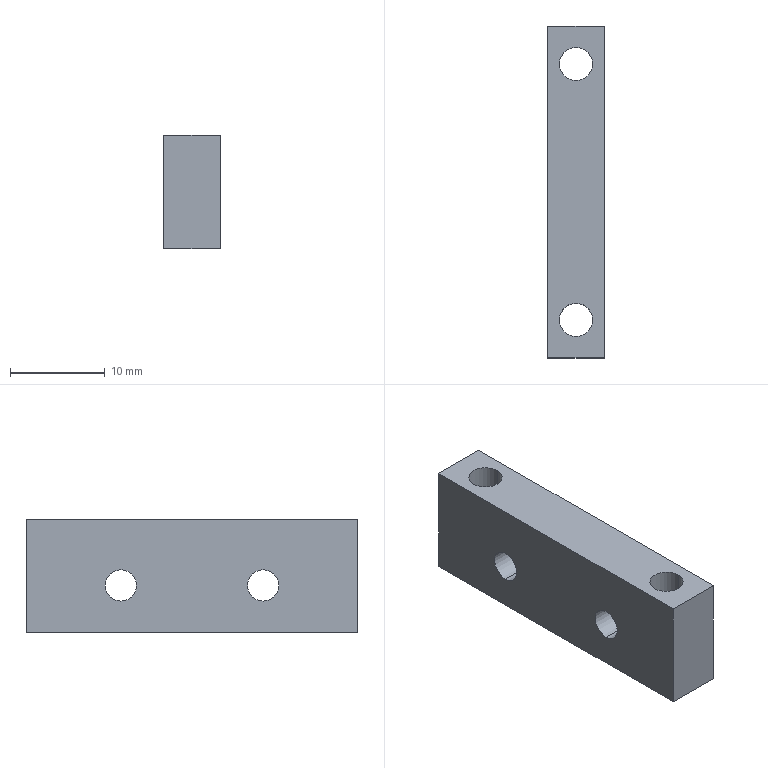Part | STEP file | Belt tensioner seat 1001 | 1 solid | 14 faces | box 6 x 35 x 12 mm | volume 2186 mm3 | cylinder 8 | plane 6 | commonest cylinder face diameters 3.3 x4 3.5 x4
STEP:
#1=CARTESIAN_POINT('',(0.,0.,0.));
#2=DIRECTION('',(0.,0.,1.));
#3=DIRECTION('',(1.,0.,0.));
#4=AXIS2_PLACEMENT_3D('',#1,#2,#3);
#5=CARTESIAN_POINT('',(0.,7.5,-8.65));
#6=VERTEX_POINT('',#5);
#7=CARTESIAN_POINT('',(6.,7.5,-8.65));
#8=VERTEX_POINT('',#7);
#9=CARTESIAN_POINT('',(6.,7.5,-8.65));
#10=DIRECTION('',(1.,0.,0.));
#11=VECTOR('',#10,1.);
#12=LINE('',#9,#11);
#13=CARTESIAN_POINT('',(6.,7.5,-7.));
#14=DIRECTION('',(1.,0.,0.));
#15=DIRECTION('',(0.,0.,-1.));
#16=AXIS2_PLACEMENT_3D('',#13,#14,#15);
#17=CYLINDRICAL_SURFACE('',#16,1.65);
#18=CARTESIAN_POINT('',(6.283,0.));
#19=DIRECTION('',(0.,1.));
#20=VECTOR('',#19,1.);
#21=LINE('',#18,#20);
#22=(GEOMETRIC_REPRESENTATION_CONTEXT(2)PARAMETRIC_REPRESENTATION_CONTEXT()REPRESENTATION_CONTEXT('',''));
#23=DEFINITIONAL_REPRESENTATION('',(#21),#22);
#24=PCURVE('',#17,#23);
#25=CARTESIAN_POINT('',(6.,7.5,-7.));
#26=DIRECTION('',(1.,0.,0.));
#27=DIRECTION('',(0.,0.,-1.));
#28=AXIS2_PLACEMENT_3D('',#25,#26,#27);
#29=CYLINDRICAL_SURFACE('',#28,1.65);
#30=CARTESIAN_POINT('',(0.,0.));
#31=DIRECTION('',(0.,1.));
#32=VECTOR('',#31,1.);
#33=LINE('',#30,#32);
#34=(GEOMETRIC_REPRESENTATION_CONTEXT(2)PARAMETRIC_REPRESENTATION_CONTEXT()REPRESENTATION_CONTEXT('',''));
#35=DEFINITIONAL_REPRESENTATION('',(#33),#34);
#36=PCURVE('',#29,#35);
#37=SURFACE_CURVE('',#12,(#24,#36),.PCURVE_S1.);
#38=EDGE_CURVE('',#6,#8,#37,.T.);
#39=ORIENTED_EDGE('',*,*,#38,.T.);
#40=CARTESIAN_POINT('',(6.,7.5,-5.35));
#41=VERTEX_POINT('',#40);
#42=CARTESIAN_POINT('',(6.,7.5,-7.));
#43=DIRECTION('',(1.,0.,0.));
#44=DIRECTION('',(0.,0.,-1.));
#45=AXIS2_PLACEMENT_3D('',#42,#43,#44);
#46=CIRCLE('',#45,1.65);
#47=CARTESIAN_POINT('',(0.,0.));
#48=DIRECTION('',(1.,0.));
#49=VECTOR('',#48,1.);
#50=LINE('',#47,#49);
#51=(GEOMETRIC_REPRESENTATION_CONTEXT(2)PARAMETRIC_REPRESENTATION_CONTEXT()REPRESENTATION_CONTEXT('',''));
#52=DEFINITIONAL_REPRESENTATION('',(#50),#51);
#53=PCURVE('',#17,#52);
#54=CARTESIAN_POINT('',(6.,17.5,-12.));
#55=DIRECTION('',(1.,0.,0.));
#56=DIRECTION('',(0.,0.,-1.));
#57=AXIS2_PLACEMENT_3D('',#54,#55,#56);
#58=PLANE('',#57);
#59=CARTESIAN_POINT('',(-5.,-10.));
#60=DIRECTION('',(1.,0.));
#61=AXIS2_PLACEMENT_2D('',#59,#60);
#62=CIRCLE('',#61,1.65);
#63=(GEOMETRIC_REPRESENTATION_CONTEXT(2)PARAMETRIC_REPRESENTATION_CONTEXT()REPRESENTATION_CONTEXT('',''));
#64=DEFINITIONAL_REPRESENTATION('',(#62),#63);
#65=PCURVE('',#58,#64);
#66=SURFACE_CURVE('',#46,(#53,#65),.PCURVE_S1.);
#67=EDGE_CURVE('',#41,#8,#66,.T.);
#68=ORIENTED_EDGE('',*,*,#67,.F.);
#69=CARTESIAN_POINT('',(0.,7.5,-5.35));
#70=VERTEX_POINT('',#69);
#71=CARTESIAN_POINT('',(6.,7.5,-5.35));
#72=DIRECTION('',(1.,0.,0.));
#73=VECTOR('',#72,1.);
#74=LINE('',#71,#73);
#75=CARTESIAN_POINT('',(3.142,0.));
#76=DIRECTION('',(0.,1.));
#77=VECTOR('',#76,1.);
#78=LINE('',#75,#77);
#79=(GEOMETRIC_REPRESENTATION_CONTEXT(2)PARAMETRIC_REPRESENTATION_CONTEXT()REPRESENTATION_CONTEXT('',''));
#80=DEFINITIONAL_REPRESENTATION('',(#78),#79);
#81=PCURVE('',#17,#80);
#82=CARTESIAN_POINT('',(3.142,0.));
#83=DIRECTION('',(0.,1.));
#84=VECTOR('',#83,1.);
#85=LINE('',#82,#84);
#86=(GEOMETRIC_REPRESENTATION_CONTEXT(2)PARAMETRIC_REPRESENTATION_CONTEXT()REPRESENTATION_CONTEXT('',''));
#87=DEFINITIONAL_REPRESENTATION('',(#85),#86);
#88=PCURVE('',#29,#87);
#89=SURFACE_CURVE('',#74,(#81,#88),.PCURVE_S1.);
#90=EDGE_CURVE('',#70,#41,#89,.T.);
#91=ORIENTED_EDGE('',*,*,#90,.F.);
#92=CARTESIAN_POINT('',(0.,7.5,-7.));
#93=DIRECTION('',(-1.,0.,0.));
#94=DIRECTION('',(0.,0.,1.));
#95=AXIS2_PLACEMENT_3D('',#92,#93,#94);
#96=CIRCLE('',#95,1.65);
#97=CARTESIAN_POINT('',(9.425,-6.));
#98=DIRECTION('',(-1.,0.));
#99=VECTOR('',#98,1.);
#100=LINE('',#97,#99);
#101=(GEOMETRIC_REPRESENTATION_CONTEXT(2)PARAMETRIC_REPRESENTATION_CONTEXT()REPRESENTATION_CONTEXT('',''));
#102=DEFINITIONAL_REPRESENTATION('',(#100),#101);
#103=PCURVE('',#17,#102);
#104=CARTESIAN_POINT('',(0.,17.5,0.));
#105=DIRECTION('',(-1.,0.,0.));
#106=DIRECTION('',(0.,0.,1.));
#107=AXIS2_PLACEMENT_3D('',#104,#105,#106);
#108=PLANE('',#107);
#109=CARTESIAN_POINT('',(-7.,-10.));
#110=DIRECTION('',(1.,0.));
#111=AXIS2_PLACEMENT_2D('',#109,#110);
#112=CIRCLE('',#111,1.65);
#113=(GEOMETRIC_REPRESENTATION_CONTEXT(2)PARAMETRIC_REPRESENTATION_CONTEXT()REPRESENTATION_CONTEXT('',''));
#114=DEFINITIONAL_REPRESENTATION('',(#112),#113);
#115=PCURVE('',#108,#114);
#116=SURFACE_CURVE('',#96,(#103,#115),.PCURVE_S1.);
#117=EDGE_CURVE('',#6,#70,#116,.T.);
#118=ORIENTED_EDGE('',*,*,#117,.F.);
#119=EDGE_LOOP('',(#39,#68,#91,#118));
#120=FACE_BOUND('',#119,.F.);
#121=ADVANCED_FACE('',(#120),#17,.F.);
#122=CARTESIAN_POINT('',(0.,-7.5,-8.65));
#123=VERTEX_POINT('',#122);
#124=CARTESIAN_POINT('',(6.,-7.5,-8.65));
#125=VERTEX_POINT('',#124);
#126=CARTESIAN_POINT('',(6.,-7.5,-8.65));
#127=DIRECTION('',(1.,0.,0.));
#128=VECTOR('',#127,1.);
#129=LINE('',#126,#128);
#130=CARTESIAN_POINT('',(6.,-7.5,-7.));
#131=DIRECTION('',(1.,0.,0.));
#132=DIRECTION('',(0.,0.,-1.));
#133=AXIS2_PLACEMENT_3D('',#130,#131,#132);
#134=CYLINDRICAL_SURFACE('',#133,1.65);
#135=CARTESIAN_POINT('',(6.283,0.));
#136=DIRECTION('',(0.,1.));
#137=VECTOR('',#136,1.);
#138=LINE('',#135,#137);
#139=(GEOMETRIC_REPRESENTATION_CONTEXT(2)PARAMETRIC_REPRESENTATION_CONTEXT()REPRESENTATION_CONTEXT('',''));
#140=DEFINITIONAL_REPRESENTATION('',(#138),#139);
#141=PCURVE('',#134,#140);
#142=CARTESIAN_POINT('',(6.,-7.5,-7.));
#143=DIRECTION('',(1.,0.,0.));
#144=DIRECTION('',(0.,0.,-1.));
#145=AXIS2_PLACEMENT_3D('',#142,#143,#144);
#146=CYLINDRICAL_SURFACE('',#145,1.65);
#147=CARTESIAN_POINT('',(0.,0.));
#148=DIRECTION('',(0.,1.));
#149=VECTOR('',#148,1.);
#150=LINE('',#147,#149);
#151=(GEOMETRIC_REPRESENTATION_CONTEXT(2)PARAMETRIC_REPRESENTATION_CONTEXT()REPRESENTATION_CONTEXT('',''));
#152=DEFINITIONAL_REPRESENTATION('',(#150),#151);
#153=PCURVE('',#146,#152);
#154=SURFACE_CURVE('',#129,(#141,#153),.PCURVE_S1.);
#155=EDGE_CURVE('',#123,#125,#154,.T.);
#156=ORIENTED_EDGE('',*,*,#155,.T.);
#157=CARTESIAN_POINT('',(6.,-7.5,-5.35));
#158=VERTEX_POINT('',#157);
#159=CARTESIAN_POINT('',(6.,-7.5,-7.));
#160=DIRECTION('',(1.,0.,0.));
#161=DIRECTION('',(0.,0.,-1.));
#162=AXIS2_PLACEMENT_3D('',#159,#160,#161);
#163=CIRCLE('',#162,1.65);
#164=CARTESIAN_POINT('',(0.,0.));
#165=DIRECTION('',(1.,0.));
#166=VECTOR('',#165,1.);
#167=LINE('',#164,#166);
#168=(GEOMETRIC_REPRESENTATION_CONTEXT(2)PARAMETRIC_REPRESENTATION_CONTEXT()REPRESENTATION_CONTEXT('',''));
#169=DEFINITIONAL_REPRESENTATION('',(#167),#168);
#170=PCURVE('',#134,#169);
#171=CARTESIAN_POINT('',(-5.,-25.));
#172=DIRECTION('',(1.,0.));
#173=AXIS2_PLACEMENT_2D('',#171,#172);
#174=CIRCLE('',#173,1.65);
#175=(GEOMETRIC_REPRESENTATION_CONTEXT(2)PARAMETRIC_REPRESENTATION_CONTEXT()REPRESENTATION_CONTEXT('',''));
#176=DEFINITIONAL_REPRESENTATION('',(#174),#175);
#177=PCURVE('',#58,#176);
#178=SURFACE_CURVE('',#163,(#170,#177),.PCURVE_S1.);
#179=EDGE_CURVE('',#158,#125,#178,.T.);
#180=ORIENTED_EDGE('',*,*,#179,.F.);
#181=CARTESIAN_POINT('',(0.,-7.5,-5.35));
#182=VERTEX_POINT('',#181);
#183=CARTESIAN_POINT('',(6.,-7.5,-5.35));
#184=DIRECTION('',(1.,0.,0.));
#185=VECTOR('',#184,1.);
#186=LINE('',#183,#185);
#187=CARTESIAN_POINT('',(3.142,0.));
#188=DIRECTION('',(0.,1.));
#189=VECTOR('',#188,1.);
#190=LINE('',#187,#189);
#191=(GEOMETRIC_REPRESENTATION_CONTEXT(2)PARAMETRIC_REPRESENTATION_CONTEXT()REPRESENTATION_CONTEXT('',''));
#192=DEFINITIONAL_REPRESENTATION('',(#190),#191);
#193=PCURVE('',#134,#192);
#194=CARTESIAN_POINT('',(3.142,0.));
#195=DIRECTION('',(0.,1.));
#196=VECTOR('',#195,1.);
#197=LINE('',#194,#196);
#198=(GEOMETRIC_REPRESENTATION_CONTEXT(2)PARAMETRIC_REPRESENTATION_CONTEXT()REPRESENTATION_CONTEXT('',''));
#199=DEFINITIONAL_REPRESENTATION('',(#197),#198);
#200=PCURVE('',#146,#199);
#201=SURFACE_CURVE('',#186,(#193,#200),.PCURVE_S1.);
#202=EDGE_CURVE('',#182,#158,#201,.T.);
#203=ORIENTED_EDGE('',*,*,#202,.F.);
#204=CARTESIAN_POINT('',(0.,-7.5,-7.));
#205=DIRECTION('',(-1.,0.,0.));
#206=DIRECTION('',(0.,0.,1.));
#207=AXIS2_PLACEMENT_3D('',#204,#205,#206);
#208=CIRCLE('',#207,1.65);
#209=CARTESIAN_POINT('',(9.425,-6.));
#210=DIRECTION('',(-1.,0.));
#211=VECTOR('',#210,1.);
#212=LINE('',#209,#211);
#213=(GEOMETRIC_REPRESENTATION_CONTEXT(2)PARAMETRIC_REPRESENTATION_CONTEXT()REPRESENTATION_CONTEXT('',''));
#214=DEFINITIONAL_REPRESENTATION('',(#212),#213);
#215=PCURVE('',#134,#214);
#216=CARTESIAN_POINT('',(-7.,-25.));
#217=DIRECTION('',(1.,0.));
#218=AXIS2_PLACEMENT_2D('',#216,#217);
#219=CIRCLE('',#218,1.65);
#220=(GEOMETRIC_REPRESENTATION_CONTEXT(2)PARAMETRIC_REPRESENTATION_CONTEXT()REPRESENTATION_CONTEXT('',''));
#221=DEFINITIONAL_REPRESENTATION('',(#219),#220);
#222=PCURVE('',#108,#221);
#223=SURFACE_CURVE('',#208,(#215,#222),.PCURVE_S1.);
#224=EDGE_CURVE('',#123,#182,#223,.T.);
#225=ORIENTED_EDGE('',*,*,#224,.F.);
#226=EDGE_LOOP('',(#156,#180,#203,#225));
#227=FACE_BOUND('',#226,.F.);
#228=ADVANCED_FACE('',(#227),#134,.F.);
#229=CARTESIAN_POINT('',(4.75,13.5,-12.));
#230=VERTEX_POINT('',#229);
#231=CARTESIAN_POINT('',(4.75,13.5,0.));
#232=VERTEX_POINT('',#231);
#233=CARTESIAN_POINT('',(4.75,13.5,-12.));
#234=DIRECTION('',(0.,0.,1.));
#235=VECTOR('',#234,1.);
#236=LINE('',#233,#235);
#237=CARTESIAN_POINT('',(3.,13.5,-12.));
#238=DIRECTION('',(0.,0.,1.));
#239=DIRECTION('',(1.,0.,0.));
#240=AXIS2_PLACEMENT_3D('',#237,#238,#239);
#241=CYLINDRICAL_SURFACE('',#240,1.75);
#242=CARTESIAN_POINT('',(6.283,0.));
#243=DIRECTION('',(0.,1.));
#244=VECTOR('',#243,1.);
#245=LINE('',#242,#244);
#246=(GEOMETRIC_REPRESENTATION_CONTEXT(2)PARAMETRIC_REPRESENTATION_CONTEXT()REPRESENTATION_CONTEXT('',''));
#247=DEFINITIONAL_REPRESENTATION('',(#245),#246);
#248=PCURVE('',#241,#247);
#249=CARTESIAN_POINT('',(3.,13.5,-12.));
#250=DIRECTION('',(0.,0.,1.));
#251=DIRECTION('',(1.,0.,0.));
#252=AXIS2_PLACEMENT_3D('',#249,#250,#251);
#253=CYLINDRICAL_SURFACE('',#252,1.75);
#254=CARTESIAN_POINT('',(0.,0.));
#255=DIRECTION('',(0.,1.));
#256=VECTOR('',#255,1.);
#257=LINE('',#254,#256);
#258=(GEOMETRIC_REPRESENTATION_CONTEXT(2)PARAMETRIC_REPRESENTATION_CONTEXT()REPRESENTATION_CONTEXT('',''));
#259=DEFINITIONAL_REPRESENTATION('',(#257),#258);
#260=PCURVE('',#253,#259);
#261=SURFACE_CURVE('',#236,(#248,#260),.PCURVE_S1.);
#262=EDGE_CURVE('',#230,#232,#261,.T.);
#263=ORIENTED_EDGE('',*,*,#262,.T.);
#264=CARTESIAN_POINT('',(1.25,13.5,0.));
#265=VERTEX_POINT('',#264);
#266=CARTESIAN_POINT('',(3.,13.5,0.));
#267=DIRECTION('',(0.,0.,1.));
#268=DIRECTION('',(1.,0.,0.));
#269=AXIS2_PLACEMENT_3D('',#266,#267,#268);
#270=CIRCLE('',#269,1.75);
#271=CARTESIAN_POINT('',(0.,12.));
#272=DIRECTION('',(1.,0.));
#273=VECTOR('',#272,1.);
#274=LINE('',#271,#273);
#275=(GEOMETRIC_REPRESENTATION_CONTEXT(2)PARAMETRIC_REPRESENTATION_CONTEXT()REPRESENTATION_CONTEXT('',''));
#276=DEFINITIONAL_REPRESENTATION('',(#274),#275);
#277=PCURVE('',#241,#276);
#278=CARTESIAN_POINT('',(0.,17.5,0.));
#279=DIRECTION('',(0.,0.,-1.));
#280=DIRECTION('',(-1.,0.,0.));
#281=AXIS2_PLACEMENT_3D('',#278,#279,#280);
#282=PLANE('',#281);
#283=CARTESIAN_POINT('',(-4.75,-4.));
#284=CARTESIAN_POINT('',(-4.75,-0.9689));
#285=CARTESIAN_POINT('',(-2.125,-2.484));
#286=CARTESIAN_POINT('',(0.5,-4.));
#287=CARTESIAN_POINT('',(-2.125,-5.516));
#288=CARTESIAN_POINT('',(-4.75,-7.031));
#289=CARTESIAN_POINT('',(-4.75,-4.));
#290=(BOUNDED_CURVE()B_SPLINE_CURVE(2,(#283,#284,#285,#286,#287,#288,#289),.UNSPECIFIED.,.T.,.F.)B_SPLINE_CURVE_WITH_KNOTS((1,2,2,2,2,1),(-2.094,0.,2.094,4.189,6.283,8.378),.UNSPECIFIED.)CURVE()GEOMETRIC_REPRESENTATION_ITEM()RATIONAL_B_SPLINE_CURVE((1.,0.5,1.,0.5,1.,0.5,1.))REPRESENTATION_ITEM(''));
#291=(GEOMETRIC_REPRESENTATION_CONTEXT(2)PARAMETRIC_REPRESENTATION_CONTEXT()REPRESENTATION_CONTEXT('',''));
#292=DEFINITIONAL_REPRESENTATION('',(#290),#291);
#293=PCURVE('',#282,#292);
#294=SURFACE_CURVE('',#270,(#277,#293),.PCURVE_S1.);
#295=EDGE_CURVE('',#265,#232,#294,.T.);
#296=ORIENTED_EDGE('',*,*,#295,.F.);
#297=CARTESIAN_POINT('',(1.25,13.5,-12.));
#298=VERTEX_POINT('',#297);
#299=CARTESIAN_POINT('',(1.25,13.5,-12.));
#300=DIRECTION('',(0.,0.,1.));
#301=VECTOR('',#300,1.);
#302=LINE('',#299,#301);
#303=CARTESIAN_POINT('',(3.142,0.));
#304=DIRECTION('',(0.,1.));
#305=VECTOR('',#304,1.);
#306=LINE('',#303,#305);
#307=(GEOMETRIC_REPRESENTATION_CONTEXT(2)PARAMETRIC_REPRESENTATION_CONTEXT()REPRESENTATION_CONTEXT('',''));
#308=DEFINITIONAL_REPRESENTATION('',(#306),#307);
#309=PCURVE('',#241,#308);
#310=CARTESIAN_POINT('',(3.142,0.));
#311=DIRECTION('',(0.,1.));
#312=VECTOR('',#311,1.);
#313=LINE('',#310,#312);
#314=(GEOMETRIC_REPRESENTATION_CONTEXT(2)PARAMETRIC_REPRESENTATION_CONTEXT()REPRESENTATION_CONTEXT('',''));
#315=DEFINITIONAL_REPRESENTATION('',(#313),#314);
#316=PCURVE('',#253,#315);
#317=SURFACE_CURVE('',#302,(#309,#316),.PCURVE_S1.);
#318=EDGE_CURVE('',#298,#265,#317,.T.);
#319=ORIENTED_EDGE('',*,*,#318,.F.);
#320=CARTESIAN_POINT('',(3.,13.5,-12.));
#321=DIRECTION('',(0.,0.,1.));
#322=DIRECTION('',(1.,0.,0.));
#323=AXIS2_PLACEMENT_3D('',#320,#321,#322);
#324=CIRCLE('',#323,1.75);
#325=CARTESIAN_POINT('',(0.,0.));
#326=DIRECTION('',(1.,0.));
#327=VECTOR('',#326,1.);
#328=LINE('',#325,#327);
#329=(GEOMETRIC_REPRESENTATION_CONTEXT(2)PARAMETRIC_REPRESENTATION_CONTEXT()REPRESENTATION_CONTEXT('',''));
#330=DEFINITIONAL_REPRESENTATION('',(#328),#329);
#331=PCURVE('',#241,#330);
#332=CARTESIAN_POINT('',(0.,17.5,-12.));
#333=DIRECTION('',(0.,0.,-1.));
#334=DIRECTION('',(-1.,0.,0.));
#335=AXIS2_PLACEMENT_3D('',#332,#333,#334);
#336=PLANE('',#335);
#337=CARTESIAN_POINT('',(-4.75,-4.));
#338=CARTESIAN_POINT('',(-4.75,-0.9689));
#339=CARTESIAN_POINT('',(-2.125,-2.484));
#340=CARTESIAN_POINT('',(0.5,-4.));
#341=CARTESIAN_POINT('',(-2.125,-5.516));
#342=CARTESIAN_POINT('',(-4.75,-7.031));
#343=CARTESIAN_POINT('',(-4.75,-4.));
#344=(BOUNDED_CURVE()B_SPLINE_CURVE(2,(#337,#338,#339,#340,#341,#342,#343),.UNSPECIFIED.,.T.,.F.)B_SPLINE_CURVE_WITH_KNOTS((1,2,2,2,2,1),(-2.094,0.,2.094,4.189,6.283,8.378),.UNSPECIFIED.)CURVE()GEOMETRIC_REPRESENTATION_ITEM()RATIONAL_B_SPLINE_CURVE((1.,0.5,1.,0.5,1.,0.5,1.))REPRESENTATION_ITEM(''));
#345=(GEOMETRIC_REPRESENTATION_CONTEXT(2)PARAMETRIC_REPRESENTATION_CONTEXT()REPRESENTATION_CONTEXT('',''));
#346=DEFINITIONAL_REPRESENTATION('',(#344),#345);
#347=PCURVE('',#336,#346);
#348=SURFACE_CURVE('',#324,(#331,#347),.PCURVE_S1.);
#349=EDGE_CURVE('',#298,#230,#348,.T.);
#350=ORIENTED_EDGE('',*,*,#349,.T.);
#351=EDGE_LOOP('',(#263,#296,#319,#350));
#352=FACE_BOUND('',#351,.F.);
#353=ADVANCED_FACE('',(#352),#241,.F.);
#354=CARTESIAN_POINT('',(4.75,-13.5,-12.));
#355=VERTEX_POINT('',#354);
#356=CARTESIAN_POINT('',(4.75,-13.5,0.));
#357=VERTEX_POINT('',#356);
#358=CARTESIAN_POINT('',(4.75,-13.5,-12.));
#359=DIRECTION('',(0.,0.,1.));
#360=VECTOR('',#359,1.);
#361=LINE('',#358,#360);
#362=CARTESIAN_POINT('',(3.,-13.5,-12.));
#363=DIRECTION('',(0.,0.,1.));
#364=DIRECTION('',(1.,0.,0.));
#365=AXIS2_PLACEMENT_3D('',#362,#363,#364);
#366=CYLINDRICAL_SURFACE('',#365,1.75);
#367=CARTESIAN_POINT('',(6.283,0.));
#368=DIRECTION('',(0.,1.));
#369=VECTOR('',#368,1.);
#370=LINE('',#367,#369);
#371=(GEOMETRIC_REPRESENTATION_CONTEXT(2)PARAMETRIC_REPRESENTATION_CONTEXT()REPRESENTATION_CONTEXT('',''));
#372=DEFINITIONAL_REPRESENTATION('',(#370),#371);
#373=PCURVE('',#366,#372);
#374=CARTESIAN_POINT('',(3.,-13.5,-12.));
#375=DIRECTION('',(0.,0.,1.));
#376=DIRECTION('',(1.,0.,0.));
#377=AXIS2_PLACEMENT_3D('',#374,#375,#376);
#378=CYLINDRICAL_SURFACE('',#377,1.75);
#379=CARTESIAN_POINT('',(0.,0.));
#380=DIRECTION('',(0.,1.));
#381=VECTOR('',#380,1.);
#382=LINE('',#379,#381);
#383=(GEOMETRIC_REPRESENTATION_CONTEXT(2)PARAMETRIC_REPRESENTATION_CONTEXT()REPRESENTATION_CONTEXT('',''));
#384=DEFINITIONAL_REPRESENTATION('',(#382),#383);
#385=PCURVE('',#378,#384);
#386=SURFACE_CURVE('',#361,(#373,#385),.PCURVE_S1.);
#387=EDGE_CURVE('',#355,#357,#386,.T.);
#388=ORIENTED_EDGE('',*,*,#387,.T.);
#389=CARTESIAN_POINT('',(1.25,-13.5,0.));
#390=VERTEX_POINT('',#389);
#391=CARTESIAN_POINT('',(3.,-13.5,0.));
#392=DIRECTION('',(0.,0.,1.));
#393=DIRECTION('',(-1.,0.,0.));
#394=AXIS2_PLACEMENT_3D('',#391,#392,#393);
#395=CIRCLE('',#394,1.75);
#396=CARTESIAN_POINT('',(3.142,12.));
#397=DIRECTION('',(1.,0.));
#398=VECTOR('',#397,1.);
#399=LINE('',#396,#398);
#400=(GEOMETRIC_REPRESENTATION_CONTEXT(2)PARAMETRIC_REPRESENTATION_CONTEXT()REPRESENTATION_CONTEXT('',''));
#401=DEFINITIONAL_REPRESENTATION('',(#399),#400);
#402=PCURVE('',#366,#401);
#403=CARTESIAN_POINT('',(-1.25,-31.));
#404=CARTESIAN_POINT('',(-1.25,-34.031));
#405=CARTESIAN_POINT('',(-3.875,-32.516));
#406=CARTESIAN_POINT('',(-6.5,-31.));
#407=CARTESIAN_POINT('',(-3.875,-29.484));
#408=CARTESIAN_POINT('',(-1.25,-27.969));
#409=CARTESIAN_POINT('',(-1.25,-31.));
#410=(BOUNDED_CURVE()B_SPLINE_CURVE(2,(#403,#404,#405,#406,#407,#408,#409),.UNSPECIFIED.,.T.,.F.)B_SPLINE_CURVE_WITH_KNOTS((1,2,2,2,2,1),(-2.094,0.,2.094,4.189,6.283,8.378),.UNSPECIFIED.)CURVE()GEOMETRIC_REPRESENTATION_ITEM()RATIONAL_B_SPLINE_CURVE((1.,0.5,1.,0.5,1.,0.5,1.))REPRESENTATION_ITEM(''));
#411=(GEOMETRIC_REPRESENTATION_CONTEXT(2)PARAMETRIC_REPRESENTATION_CONTEXT()REPRESENTATION_CONTEXT('',''));
#412=DEFINITIONAL_REPRESENTATION('',(#410),#411);
#413=PCURVE('',#282,#412);
#414=SURFACE_CURVE('',#395,(#402,#413),.PCURVE_S1.);
#415=EDGE_CURVE('',#390,#357,#414,.T.);
#416=ORIENTED_EDGE('',*,*,#415,.F.);
#417=CARTESIAN_POINT('',(1.25,-13.5,-12.));
#418=VERTEX_POINT('',#417);
#419=CARTESIAN_POINT('',(1.25,-13.5,-12.));
#420=DIRECTION('',(0.,0.,1.));
#421=VECTOR('',#420,1.);
#422=LINE('',#419,#421);
#423=CARTESIAN_POINT('',(3.142,0.));
#424=DIRECTION('',(0.,1.));
#425=VECTOR('',#424,1.);
#426=LINE('',#423,#425);
#427=(GEOMETRIC_REPRESENTATION_CONTEXT(2)PARAMETRIC_REPRESENTATION_CONTEXT()REPRESENTATION_CONTEXT('',''));
#428=DEFINITIONAL_REPRESENTATION('',(#426),#427);
#429=PCURVE('',#366,#428);
#430=CARTESIAN_POINT('',(3.142,0.));
#431=DIRECTION('',(0.,1.));
#432=VECTOR('',#431,1.);
#433=LINE('',#430,#432);
#434=(GEOMETRIC_REPRESENTATION_CONTEXT(2)PARAMETRIC_REPRESENTATION_CONTEXT()REPRESENTATION_CONTEXT('',''));
#435=DEFINITIONAL_REPRESENTATION('',(#433),#434);
#436=PCURVE('',#378,#435);
#437=SURFACE_CURVE('',#422,(#429,#436),.PCURVE_S1.);
#438=EDGE_CURVE('',#418,#390,#437,.T.);
#439=ORIENTED_EDGE('',*,*,#438,.F.);
#440=CARTESIAN_POINT('',(3.,-13.5,-12.));
#441=DIRECTION('',(0.,0.,1.));
#442=DIRECTION('',(-1.,0.,0.));
#443=AXIS2_PLACEMENT_3D('',#440,#441,#442);
#444=CIRCLE('',#443,1.75);
#445=CARTESIAN_POINT('',(3.142,0.));
#446=DIRECTION('',(1.,0.));
#447=VECTOR('',#446,1.);
#448=LINE('',#445,#447);
#449=(GEOMETRIC_REPRESENTATION_CONTEXT(2)PARAMETRIC_REPRESENTATION_CONTEXT()REPRESENTATION_CONTEXT('',''));
#450=DEFINITIONAL_REPRESENTATION('',(#448),#449);
#451=PCURVE('',#366,#450);
#452=CARTESIAN_POINT('',(-1.25,-31.));
#453=CARTESIAN_POINT('',(-1.25,-34.031));
#454=CARTESIAN_POINT('',(-3.875,-32.516));
#455=CARTESIAN_POINT('',(-6.5,-31.));
#456=CARTESIAN_POINT('',(-3.875,-29.484));
#457=CARTESIAN_POINT('',(-1.25,-27.969));
#458=CARTESIAN_POINT('',(-1.25,-31.));
#459=(BOUNDED_CURVE()B_SPLINE_CURVE(2,(#452,#453,#454,#455,#456,#457,#458),.UNSPECIFIED.,.T.,.F.)B_SPLINE_CURVE_WITH_KNOTS((1,2,2,2,2,1),(-2.094,0.,2.094,4.189,6.283,8.378),.UNSPECIFIED.)CURVE()GEOMETRIC_REPRESENTATION_ITEM()RATIONAL_B_SPLINE_CURVE((1.,0.5,1.,0.5,1.,0.5,1.))REPRESENTATION_ITEM(''));
#460=(GEOMETRIC_REPRESENTATION_CONTEXT(2)PARAMETRIC_REPRESENTATION_CONTEXT()REPRESENTATION_CONTEXT('',''));
#461=DEFINITIONAL_REPRESENTATION('',(#459),#460);
#462=PCURVE('',#336,#461);
#463=SURFACE_CURVE('',#444,(#451,#462),.PCURVE_S1.);
#464=EDGE_CURVE('',#418,#355,#463,.T.);
#465=ORIENTED_EDGE('',*,*,#464,.T.);
#466=EDGE_LOOP('',(#388,#416,#439,#465));
#467=FACE_BOUND('',#466,.F.);
#468=ADVANCED_FACE('',(#467),#366,.F.);
#469=CARTESIAN_POINT('',(3.,13.5,0.));
#470=DIRECTION('',(0.,0.,1.));
#471=DIRECTION('',(1.,0.,0.));
#472=AXIS2_PLACEMENT_3D('',#469,#470,#471);
#473=CIRCLE('',#472,1.75);
#474=CARTESIAN_POINT('',(-4.75,-4.));
#475=CARTESIAN_POINT('',(-4.75,-0.9689));
#476=CARTESIAN_POINT('',(-2.125,-2.484));
#477=CARTESIAN_POINT('',(0.5,-4.));
#478=CARTESIAN_POINT('',(-2.125,-5.516));
#479=CARTESIAN_POINT('',(-4.75,-7.031));
#480=CARTESIAN_POINT('',(-4.75,-4.));
#481=(BOUNDED_CURVE()B_SPLINE_CURVE(2,(#474,#475,#476,#477,#478,#479,#480),.UNSPECIFIED.,.T.,.F.)B_SPLINE_CURVE_WITH_KNOTS((1,2,2,2,2,1),(-2.094,0.,2.094,4.189,6.283,8.378),.UNSPECIFIED.)CURVE()GEOMETRIC_REPRESENTATION_ITEM()RATIONAL_B_SPLINE_CURVE((1.,0.5,1.,0.5,1.,0.5,1.))REPRESENTATION_ITEM(''));
#482=(GEOMETRIC_REPRESENTATION_CONTEXT(2)PARAMETRIC_REPRESENTATION_CONTEXT()REPRESENTATION_CONTEXT('',''));
#483=DEFINITIONAL_REPRESENTATION('',(#481),#482);
#484=PCURVE('',#282,#483);
#485=CARTESIAN_POINT('',(0.,12.));
#486=DIRECTION('',(1.,0.));
#487=VECTOR('',#486,1.);
#488=LINE('',#485,#487);
#489=(GEOMETRIC_REPRESENTATION_CONTEXT(2)PARAMETRIC_REPRESENTATION_CONTEXT()REPRESENTATION_CONTEXT('',''));
#490=DEFINITIONAL_REPRESENTATION('',(#488),#489);
#491=PCURVE('',#253,#490);
#492=SURFACE_CURVE('',#473,(#484,#491),.PCURVE_S1.);
#493=EDGE_CURVE('',#232,#265,#492,.T.);
#494=ORIENTED_EDGE('',*,*,#493,.F.);
#495=ORIENTED_EDGE('',*,*,#295,.F.);
#496=EDGE_LOOP('',(#494,#495));
#497=FACE_BOUND('',#496,.T.);
#498=CARTESIAN_POINT('',(3.,-13.5,0.));
#499=DIRECTION('',(0.,0.,1.));
#500=DIRECTION('',(-1.,0.,0.));
#501=AXIS2_PLACEMENT_3D('',#498,#499,#500);
#502=CIRCLE('',#501,1.75);
#503=CARTESIAN_POINT('',(-1.25,-31.));
#504=CARTESIAN_POINT('',(-1.25,-34.031));
#505=CARTESIAN_POINT('',(-3.875,-32.516));
#506=CARTESIAN_POINT('',(-6.5,-31.));
#507=CARTESIAN_POINT('',(-3.875,-29.484));
#508=CARTESIAN_POINT('',(-1.25,-27.969));
#509=CARTESIAN_POINT('',(-1.25,-31.));
#510=(BOUNDED_CURVE()B_SPLINE_CURVE(2,(#503,#504,#505,#506,#507,#508,#509),.UNSPECIFIED.,.T.,.F.)B_SPLINE_CURVE_WITH_KNOTS((1,2,2,2,2,1),(-2.094,0.,2.094,4.189,6.283,8.378),.UNSPECIFIED.)CURVE()GEOMETRIC_REPRESENTATION_ITEM()RATIONAL_B_SPLINE_CURVE((1.,0.5,1.,0.5,1.,0.5,1.))REPRESENTATION_ITEM(''));
#511=(GEOMETRIC_REPRESENTATION_CONTEXT(2)PARAMETRIC_REPRESENTATION_CONTEXT()REPRESENTATION_CONTEXT('',''));
#512=DEFINITIONAL_REPRESENTATION('',(#510),#511);
#513=PCURVE('',#282,#512);
#514=CARTESIAN_POINT('',(-3.142,12.));
#515=DIRECTION('',(1.,0.));
#516=VECTOR('',#515,1.);
#517=LINE('',#514,#516);
#518=(GEOMETRIC_REPRESENTATION_CONTEXT(2)PARAMETRIC_REPRESENTATION_CONTEXT()REPRESENTATION_CONTEXT('',''));
#519=DEFINITIONAL_REPRESENTATION('',(#517),#518);
#520=PCURVE('',#378,#519);
#521=SURFACE_CURVE('',#502,(#513,#520),.PCURVE_S1.);
#522=EDGE_CURVE('',#357,#390,#521,.T.);
#523=ORIENTED_EDGE('',*,*,#522,.F.);
#524=ORIENTED_EDGE('',*,*,#415,.F.);
#525=EDGE_LOOP('',(#523,#524));
#526=FACE_BOUND('',#525,.T.);
#527=CARTESIAN_POINT('',(0.,-17.5,0.));
#528=VERTEX_POINT('',#527);
#529=CARTESIAN_POINT('',(6.,-17.5,0.));
#530=VERTEX_POINT('',#529);
#531=CARTESIAN_POINT('',(0.,-17.5,0.));
#532=DIRECTION('',(1.,0.,0.));
#533=VECTOR('',#532,1.);
#534=LINE('',#531,#533);
#535=CARTESIAN_POINT('',(0.,-35.));
#536=DIRECTION('',(-1.,0.));
#537=VECTOR('',#536,1.);
#538=LINE('',#535,#537);
#539=(GEOMETRIC_REPRESENTATION_CONTEXT(2)PARAMETRIC_REPRESENTATION_CONTEXT()REPRESENTATION_CONTEXT('',''));
#540=DEFINITIONAL_REPRESENTATION('',(#538),#539);
#541=PCURVE('',#282,#540);
#542=CARTESIAN_POINT('',(0.,-17.5,0.));
#543=DIRECTION('',(0.,-1.,0.));
#544=DIRECTION('',(-1.,0.,0.));
#545=AXIS2_PLACEMENT_3D('',#542,#543,#544);
#546=PLANE('',#545);
#547=CARTESIAN_POINT('',(0.,0.));
#548=DIRECTION('',(-1.,0.));
#549=VECTOR('',#548,1.);
#550=LINE('',#547,#549);
#551=(GEOMETRIC_REPRESENTATION_CONTEXT(2)PARAMETRIC_REPRESENTATION_CONTEXT()REPRESENTATION_CONTEXT('',''));
#552=DEFINITIONAL_REPRESENTATION('',(#550),#551);
#553=PCURVE('',#546,#552);
#554=SURFACE_CURVE('',#534,(#541,#553),.PCURVE_S1.);
#555=EDGE_CURVE('',#528,#530,#554,.T.);
#556=ORIENTED_EDGE('',*,*,#555,.T.);
#557=CARTESIAN_POINT('',(6.,17.5,0.));
#558=VERTEX_POINT('',#557);
#559=CARTESIAN_POINT('',(6.,17.5,0.));
#560=DIRECTION('',(0.,-1.,0.));
#561=VECTOR('',#560,1.);
#562=LINE('',#559,#561);
#563=CARTESIAN_POINT('',(-6.,0.));
#564=DIRECTION('',(0.,-1.));
#565=VECTOR('',#564,1.);
#566=LINE('',#563,#565);
#567=(GEOMETRIC_REPRESENTATION_CONTEXT(2)PARAMETRIC_REPRESENTATION_CONTEXT()REPRESENTATION_CONTEXT('',''));
#568=DEFINITIONAL_REPRESENTATION('',(#566),#567);
#569=PCURVE('',#282,#568);
#570=CARTESIAN_POINT('',(-12.,0.));
#571=DIRECTION('',(0.,-1.));
#572=VECTOR('',#571,1.);
#573=LINE('',#570,#572);
#574=(GEOMETRIC_REPRESENTATION_CONTEXT(2)PARAMETRIC_REPRESENTATION_CONTEXT()REPRESENTATION_CONTEXT('',''));
#575=DEFINITIONAL_REPRESENTATION('',(#573),#574);
#576=PCURVE('',#58,#575);
#577=SURFACE_CURVE('',#562,(#569,#576),.PCURVE_S1.);
#578=EDGE_CURVE('',#558,#530,#577,.T.);
#579=ORIENTED_EDGE('',*,*,#578,.F.);
#580=CARTESIAN_POINT('',(0.,17.5,0.));
#581=VERTEX_POINT('',#580);
#582=CARTESIAN_POINT('',(0.,17.5,0.));
#583=DIRECTION('',(1.,0.,0.));
#584=VECTOR('',#583,1.);
#585=LINE('',#582,#584);
#586=CARTESIAN_POINT('',(0.,0.));
#587=DIRECTION('',(-1.,0.));
#588=VECTOR('',#587,1.);
#589=LINE('',#586,#588);
#590=(GEOMETRIC_REPRESENTATION_CONTEXT(2)PARAMETRIC_REPRESENTATION_CONTEXT()REPRESENTATION_CONTEXT('',''));
#591=DEFINITIONAL_REPRESENTATION('',(#589),#590);
#592=PCURVE('',#282,#591);
#593=CARTESIAN_POINT('',(0.,17.5,0.));
#594=DIRECTION('',(0.,-1.,0.));
#595=DIRECTION('',(-1.,0.,0.));
#596=AXIS2_PLACEMENT_3D('',#593,#594,#595);
#597=PLANE('',#596);
#598=CARTESIAN_POINT('',(0.,0.));
#599=DIRECTION('',(-1.,0.));
#600=VECTOR('',#599,1.);
#601=LINE('',#598,#600);
#602=(GEOMETRIC_REPRESENTATION_CONTEXT(2)PARAMETRIC_REPRESENTATION_CONTEXT()REPRESENTATION_CONTEXT('',''));
#603=DEFINITIONAL_REPRESENTATION('',(#601),#602);
#604=PCURVE('',#597,#603);
#605=SURFACE_CURVE('',#585,(#592,#604),.PCURVE_S1.);
#606=EDGE_CURVE('',#581,#558,#605,.T.);
#607=ORIENTED_EDGE('',*,*,#606,.F.);
#608=CARTESIAN_POINT('',(0.,17.5,0.));
#609=DIRECTION('',(0.,-1.,0.));
#610=VECTOR('',#609,1.);
#611=LINE('',#608,#610);
#612=CARTESIAN_POINT('',(0.,0.));
#613=DIRECTION('',(0.,-1.));
#614=VECTOR('',#613,1.);
#615=LINE('',#612,#614);
#616=(GEOMETRIC_REPRESENTATION_CONTEXT(2)PARAMETRIC_REPRESENTATION_CONTEXT()REPRESENTATION_CONTEXT('',''));
#617=DEFINITIONAL_REPRESENTATION('',(#615),#616);
#618=PCURVE('',#282,#617);
#619=CARTESIAN_POINT('',(0.,0.));
#620=DIRECTION('',(0.,-1.));
#621=VECTOR('',#620,1.);
#622=LINE('',#619,#621);
#623=(GEOMETRIC_REPRESENTATION_CONTEXT(2)PARAMETRIC_REPRESENTATION_CONTEXT()REPRESENTATION_CONTEXT('',''));
#624=DEFINITIONAL_REPRESENTATION('',(#622),#623);
#625=PCURVE('',#108,#624);
#626=SURFACE_CURVE('',#611,(#618,#625),.PCURVE_S1.);
#627=EDGE_CURVE('',#581,#528,#626,.T.);
#628=ORIENTED_EDGE('',*,*,#627,.T.);
#629=EDGE_LOOP('',(#556,#579,#607,#628));
#630=FACE_BOUND('',#629,.T.);
#631=ADVANCED_FACE('',(#497,#526,#630),#282,.F.);
#632=CARTESIAN_POINT('',(6.,7.5,-7.));
#633=DIRECTION('',(1.,0.,0.));
#634=DIRECTION('',(0.,0.,-1.));
#635=AXIS2_PLACEMENT_3D('',#632,#633,#634);
#636=CIRCLE('',#635,1.65);
#637=CARTESIAN_POINT('',(-5.,-10.));
#638=DIRECTION('',(1.,0.));
#639=AXIS2_PLACEMENT_2D('',#637,#638);
#640=CIRCLE('',#639,1.65);
#641=(GEOMETRIC_REPRESENTATION_CONTEXT(2)PARAMETRIC_REPRESENTATION_CONTEXT()REPRESENTATION_CONTEXT('',''));
#642=DEFINITIONAL_REPRESENTATION('',(#640),#641);
#643=PCURVE('',#58,#642);
#644=CARTESIAN_POINT('',(0.,0.));
#645=DIRECTION('',(1.,0.));
#646=VECTOR('',#645,1.);
#647=LINE('',#644,#646);
#648=(GEOMETRIC_REPRESENTATION_CONTEXT(2)PARAMETRIC_REPRESENTATION_CONTEXT()REPRESENTATION_CONTEXT('',''));
#649=DEFINITIONAL_REPRESENTATION('',(#647),#648);
#650=PCURVE('',#29,#649);
#651=SURFACE_CURVE('',#636,(#643,#650),.PCURVE_S1.);
#652=EDGE_CURVE('',#8,#41,#651,.T.);
#653=ORIENTED_EDGE('',*,*,#652,.F.);
#654=ORIENTED_EDGE('',*,*,#67,.F.);
#655=EDGE_LOOP('',(#653,#654));
#656=FACE_BOUND('',#655,.T.);
#657=CARTESIAN_POINT('',(6.,-7.5,-7.));
#658=DIRECTION('',(1.,0.,0.));
#659=DIRECTION('',(0.,0.,-1.));
#660=AXIS2_PLACEMENT_3D('',#657,#658,#659);
#661=CIRCLE('',#660,1.65);
#662=CARTESIAN_POINT('',(-5.,-25.));
#663=DIRECTION('',(1.,0.));
#664=AXIS2_PLACEMENT_2D('',#662,#663);
#665=CIRCLE('',#664,1.65);
#666=(GEOMETRIC_REPRESENTATION_CONTEXT(2)PARAMETRIC_REPRESENTATION_CONTEXT()REPRESENTATION_CONTEXT('',''));
#667=DEFINITIONAL_REPRESENTATION('',(#665),#666);
#668=PCURVE('',#58,#667);
#669=CARTESIAN_POINT('',(0.,0.));
#670=DIRECTION('',(1.,0.));
#671=VECTOR('',#670,1.);
#672=LINE('',#669,#671);
#673=(GEOMETRIC_REPRESENTATION_CONTEXT(2)PARAMETRIC_REPRESENTATION_CONTEXT()REPRESENTATION_CONTEXT('',''));
#674=DEFINITIONAL_REPRESENTATION('',(#672),#673);
#675=PCURVE('',#146,#674);
#676=SURFACE_CURVE('',#661,(#668,#675),.PCURVE_S1.);
#677=EDGE_CURVE('',#125,#158,#676,.T.);
#678=ORIENTED_EDGE('',*,*,#677,.F.);
#679=ORIENTED_EDGE('',*,*,#179,.F.);
#680=EDGE_LOOP('',(#678,#679));
#681=FACE_BOUND('',#680,.T.);
#682=CARTESIAN_POINT('',(6.,-17.5,-12.));
#683=VERTEX_POINT('',#682);
#684=CARTESIAN_POINT('',(6.,-17.5,-12.));
#685=DIRECTION('',(0.,0.,1.));
#686=VECTOR('',#685,1.);
#687=LINE('',#684,#686);
#688=CARTESIAN_POINT('',(0.,-35.));
#689=DIRECTION('',(-1.,0.));
#690=VECTOR('',#689,1.);
#691=LINE('',#688,#690);
#692=(GEOMETRIC_REPRESENTATION_CONTEXT(2)PARAMETRIC_REPRESENTATION_CONTEXT()REPRESENTATION_CONTEXT('',''));
#693=DEFINITIONAL_REPRESENTATION('',(#691),#692);
#694=PCURVE('',#58,#693);
#695=CARTESIAN_POINT('',(-6.,12.));
#696=DIRECTION('',(0.,-1.));
#697=VECTOR('',#696,1.);
#698=LINE('',#695,#697);
#699=(GEOMETRIC_REPRESENTATION_CONTEXT(2)PARAMETRIC_REPRESENTATION_CONTEXT()REPRESENTATION_CONTEXT('',''));
#700=DEFINITIONAL_REPRESENTATION('',(#698),#699);
#701=PCURVE('',#546,#700);
#702=SURFACE_CURVE('',#687,(#694,#701),.PCURVE_S1.);
#703=EDGE_CURVE('',#683,#530,#702,.T.);
#704=ORIENTED_EDGE('',*,*,#703,.F.);
#705=CARTESIAN_POINT('',(6.,17.5,-12.));
#706=VERTEX_POINT('',#705);
#707=CARTESIAN_POINT('',(6.,17.5,-12.));
#708=DIRECTION('',(0.,-1.,0.));
#709=VECTOR('',#708,1.);
#710=LINE('',#707,#709);
#711=CARTESIAN_POINT('',(0.,0.));
#712=DIRECTION('',(0.,-1.));
#713=VECTOR('',#712,1.);
#714=LINE('',#711,#713);
#715=(GEOMETRIC_REPRESENTATION_CONTEXT(2)PARAMETRIC_REPRESENTATION_CONTEXT()REPRESENTATION_CONTEXT('',''));
#716=DEFINITIONAL_REPRESENTATION('',(#714),#715);
#717=PCURVE('',#58,#716);
#718=CARTESIAN_POINT('',(-6.,0.));
#719=DIRECTION('',(0.,-1.));
#720=VECTOR('',#719,1.);
#721=LINE('',#718,#720);
#722=(GEOMETRIC_REPRESENTATION_CONTEXT(2)PARAMETRIC_REPRESENTATION_CONTEXT()REPRESENTATION_CONTEXT('',''));
#723=DEFINITIONAL_REPRESENTATION('',(#721),#722);
#724=PCURVE('',#336,#723);
#725=SURFACE_CURVE('',#710,(#717,#724),.PCURVE_S1.);
#726=EDGE_CURVE('',#706,#683,#725,.T.);
#727=ORIENTED_EDGE('',*,*,#726,.F.);
#728=CARTESIAN_POINT('',(6.,17.5,-12.));
#729=DIRECTION('',(0.,0.,1.));
#730=VECTOR('',#729,1.);
#731=LINE('',#728,#730);
#732=CARTESIAN_POINT('',(0.,0.));
#733=DIRECTION('',(-1.,0.));
#734=VECTOR('',#733,1.);
#735=LINE('',#732,#734);
#736=(GEOMETRIC_REPRESENTATION_CONTEXT(2)PARAMETRIC_REPRESENTATION_CONTEXT()REPRESENTATION_CONTEXT('',''));
#737=DEFINITIONAL_REPRESENTATION('',(#735),#736);
#738=PCURVE('',#58,#737);
#739=CARTESIAN_POINT('',(-6.,12.));
#740=DIRECTION('',(0.,-1.));
#741=VECTOR('',#740,1.);
#742=LINE('',#739,#741);
#743=(GEOMETRIC_REPRESENTATION_CONTEXT(2)PARAMETRIC_REPRESENTATION_CONTEXT()REPRESENTATION_CONTEXT('',''));
#744=DEFINITIONAL_REPRESENTATION('',(#742),#743);
#745=PCURVE('',#597,#744);
#746=SURFACE_CURVE('',#731,(#738,#745),.PCURVE_S1.);
#747=EDGE_CURVE('',#706,#558,#746,.T.);
#748=ORIENTED_EDGE('',*,*,#747,.T.);
#749=ORIENTED_EDGE('',*,*,#578,.T.);
#750=EDGE_LOOP('',(#704,#727,#748,#749));
#751=FACE_BOUND('',#750,.T.);
#752=ADVANCED_FACE('',(#656,#681,#751),#58,.T.);
#753=CARTESIAN_POINT('',(3.,13.5,-12.));
#754=DIRECTION('',(0.,0.,1.));
#755=DIRECTION('',(1.,0.,0.));
#756=AXIS2_PLACEMENT_3D('',#753,#754,#755);
#757=CIRCLE('',#756,1.75);
#758=CARTESIAN_POINT('',(-4.75,-4.));
#759=CARTESIAN_POINT('',(-4.75,-0.9689));
#760=CARTESIAN_POINT('',(-2.125,-2.484));
#761=CARTESIAN_POINT('',(0.5,-4.));
#762=CARTESIAN_POINT('',(-2.125,-5.516));
#763=CARTESIAN_POINT('',(-4.75,-7.031));
#764=CARTESIAN_POINT('',(-4.75,-4.));
#765=(BOUNDED_CURVE()B_SPLINE_CURVE(2,(#758,#759,#760,#761,#762,#763,#764),.UNSPECIFIED.,.T.,.F.)B_SPLINE_CURVE_WITH_KNOTS((1,2,2,2,2,1),(-2.094,0.,2.094,4.189,6.283,8.378),.UNSPECIFIED.)CURVE()GEOMETRIC_REPRESENTATION_ITEM()RATIONAL_B_SPLINE_CURVE((1.,0.5,1.,0.5,1.,0.5,1.))REPRESENTATION_ITEM(''));
#766=(GEOMETRIC_REPRESENTATION_CONTEXT(2)PARAMETRIC_REPRESENTATION_CONTEXT()REPRESENTATION_CONTEXT('',''));
#767=DEFINITIONAL_REPRESENTATION('',(#765),#766);
#768=PCURVE('',#336,#767);
#769=CARTESIAN_POINT('',(0.,0.));
#770=DIRECTION('',(1.,0.));
#771=VECTOR('',#770,1.);
#772=LINE('',#769,#771);
#773=(GEOMETRIC_REPRESENTATION_CONTEXT(2)PARAMETRIC_REPRESENTATION_CONTEXT()REPRESENTATION_CONTEXT('',''));
#774=DEFINITIONAL_REPRESENTATION('',(#772),#773);
#775=PCURVE('',#253,#774);
#776=SURFACE_CURVE('',#757,(#768,#775),.PCURVE_S1.);
#777=EDGE_CURVE('',#230,#298,#776,.T.);
#778=ORIENTED_EDGE('',*,*,#777,.T.);
#779=ORIENTED_EDGE('',*,*,#349,.T.);
#780=EDGE_LOOP('',(#778,#779));
#781=FACE_BOUND('',#780,.T.);
#782=CARTESIAN_POINT('',(3.,-13.5,-12.));
#783=DIRECTION('',(0.,0.,1.));
#784=DIRECTION('',(-1.,0.,0.));
#785=AXIS2_PLACEMENT_3D('',#782,#783,#784);
#786=CIRCLE('',#785,1.75);
#787=CARTESIAN_POINT('',(-1.25,-31.));
#788=CARTESIAN_POINT('',(-1.25,-34.031));
#789=CARTESIAN_POINT('',(-3.875,-32.516));
#790=CARTESIAN_POINT('',(-6.5,-31.));
#791=CARTESIAN_POINT('',(-3.875,-29.484));
#792=CARTESIAN_POINT('',(-1.25,-27.969));
#793=CARTESIAN_POINT('',(-1.25,-31.));
#794=(BOUNDED_CURVE()B_SPLINE_CURVE(2,(#787,#788,#789,#790,#791,#792,#793),.UNSPECIFIED.,.T.,.F.)B_SPLINE_CURVE_WITH_KNOTS((1,2,2,2,2,1),(-2.094,0.,2.094,4.189,6.283,8.378),.UNSPECIFIED.)CURVE()GEOMETRIC_REPRESENTATION_ITEM()RATIONAL_B_SPLINE_CURVE((1.,0.5,1.,0.5,1.,0.5,1.))REPRESENTATION_ITEM(''));
#795=(GEOMETRIC_REPRESENTATION_CONTEXT(2)PARAMETRIC_REPRESENTATION_CONTEXT()REPRESENTATION_CONTEXT('',''));
#796=DEFINITIONAL_REPRESENTATION('',(#794),#795);
#797=PCURVE('',#336,#796);
#798=CARTESIAN_POINT('',(-3.142,0.));
#799=DIRECTION('',(1.,0.));
#800=VECTOR('',#799,1.);
#801=LINE('',#798,#800);
#802=(GEOMETRIC_REPRESENTATION_CONTEXT(2)PARAMETRIC_REPRESENTATION_CONTEXT()REPRESENTATION_CONTEXT('',''));
#803=DEFINITIONAL_REPRESENTATION('',(#801),#802);
#804=PCURVE('',#378,#803);
#805=SURFACE_CURVE('',#786,(#797,#804),.PCURVE_S1.);
#806=EDGE_CURVE('',#355,#418,#805,.T.);
#807=ORIENTED_EDGE('',*,*,#806,.T.);
#808=ORIENTED_EDGE('',*,*,#464,.T.);
#809=EDGE_LOOP('',(#807,#808));
#810=FACE_BOUND('',#809,.T.);
#811=CARTESIAN_POINT('',(0.,-17.5,-12.));
#812=VERTEX_POINT('',#811);
#813=CARTESIAN_POINT('',(0.,-17.5,-12.));
#814=DIRECTION('',(1.,0.,0.));
#815=VECTOR('',#814,1.);
#816=LINE('',#813,#815);
#817=CARTESIAN_POINT('',(0.,-35.));
#818=DIRECTION('',(-1.,0.));
#819=VECTOR('',#818,1.);
#820=LINE('',#817,#819);
#821=(GEOMETRIC_REPRESENTATION_CONTEXT(2)PARAMETRIC_REPRESENTATION_CONTEXT()REPRESENTATION_CONTEXT('',''));
#822=DEFINITIONAL_REPRESENTATION('',(#820),#821);
#823=PCURVE('',#336,#822);
#824=CARTESIAN_POINT('',(0.,12.));
#825=DIRECTION('',(-1.,0.));
#826=VECTOR('',#825,1.);
#827=LINE('',#824,#826);
#828=(GEOMETRIC_REPRESENTATION_CONTEXT(2)PARAMETRIC_REPRESENTATION_CONTEXT()REPRESENTATION_CONTEXT('',''));
#829=DEFINITIONAL_REPRESENTATION('',(#827),#828);
#830=PCURVE('',#546,#829);
#831=SURFACE_CURVE('',#816,(#823,#830),.PCURVE_S1.);
#832=EDGE_CURVE('',#812,#683,#831,.T.);
#833=ORIENTED_EDGE('',*,*,#832,.F.);
#834=CARTESIAN_POINT('',(0.,17.5,-12.));
#835=VERTEX_POINT('',#834);
#836=CARTESIAN_POINT('',(0.,17.5,-12.));
#837=DIRECTION('',(0.,-1.,0.));
#838=VECTOR('',#837,1.);
#839=LINE('',#836,#838);
#840=CARTESIAN_POINT('',(0.,0.));
#841=DIRECTION('',(0.,-1.));
#842=VECTOR('',#841,1.);
#843=LINE('',#840,#842);
#844=(GEOMETRIC_REPRESENTATION_CONTEXT(2)PARAMETRIC_REPRESENTATION_CONTEXT()REPRESENTATION_CONTEXT('',''));
#845=DEFINITIONAL_REPRESENTATION('',(#843),#844);
#846=PCURVE('',#336,#845);
#847=CARTESIAN_POINT('',(-12.,0.));
#848=DIRECTION('',(0.,-1.));
#849=VECTOR('',#848,1.);
#850=LINE('',#847,#849);
#851=(GEOMETRIC_REPRESENTATION_CONTEXT(2)PARAMETRIC_REPRESENTATION_CONTEXT()REPRESENTATION_CONTEXT('',''));
#852=DEFINITIONAL_REPRESENTATION('',(#850),#851);
#853=PCURVE('',#108,#852);
#854=SURFACE_CURVE('',#839,(#846,#853),.PCURVE_S1.);
#855=EDGE_CURVE('',#835,#812,#854,.T.);
#856=ORIENTED_EDGE('',*,*,#855,.F.);
#857=CARTESIAN_POINT('',(0.,17.5,-12.));
#858=DIRECTION('',(1.,0.,0.));
#859=VECTOR('',#858,1.);
#860=LINE('',#857,#859);
#861=CARTESIAN_POINT('',(0.,0.));
#862=DIRECTION('',(-1.,0.));
#863=VECTOR('',#862,1.);
#864=LINE('',#861,#863);
#865=(GEOMETRIC_REPRESENTATION_CONTEXT(2)PARAMETRIC_REPRESENTATION_CONTEXT()REPRESENTATION_CONTEXT('',''));
#866=DEFINITIONAL_REPRESENTATION('',(#864),#865);
#867=PCURVE('',#336,#866);
#868=CARTESIAN_POINT('',(0.,12.));
#869=DIRECTION('',(-1.,0.));
#870=VECTOR('',#869,1.);
#871=LINE('',#868,#870);
#872=(GEOMETRIC_REPRESENTATION_CONTEXT(2)PARAMETRIC_REPRESENTATION_CONTEXT()REPRESENTATION_CONTEXT('',''));
#873=DEFINITIONAL_REPRESENTATION('',(#871),#872);
#874=PCURVE('',#597,#873);
#875=SURFACE_CURVE('',#860,(#867,#874),.PCURVE_S1.);
#876=EDGE_CURVE('',#835,#706,#875,.T.);
#877=ORIENTED_EDGE('',*,*,#876,.T.);
#878=ORIENTED_EDGE('',*,*,#726,.T.);
#879=EDGE_LOOP('',(#833,#856,#877,#878));
#880=FACE_BOUND('',#879,.T.);
#881=ADVANCED_FACE('',(#781,#810,#880),#336,.T.);
#882=ORIENTED_EDGE('',*,*,#117,.F.);
#883=CARTESIAN_POINT('',(0.,7.5,-7.));
#884=DIRECTION('',(-1.,0.,0.));
#885=DIRECTION('',(0.,0.,1.));
#886=AXIS2_PLACEMENT_3D('',#883,#884,#885);
#887=CIRCLE('',#886,1.65);
#888=CARTESIAN_POINT('',(-7.,-10.));
#889=DIRECTION('',(1.,0.));
#890=AXIS2_PLACEMENT_2D('',#888,#889);
#891=CIRCLE('',#890,1.65);
#892=(GEOMETRIC_REPRESENTATION_CONTEXT(2)PARAMETRIC_REPRESENTATION_CONTEXT()REPRESENTATION_CONTEXT('',''));
#893=DEFINITIONAL_REPRESENTATION('',(#891),#892);
#894=PCURVE('',#108,#893);
#895=CARTESIAN_POINT('',(3.142,-6.));
#896=DIRECTION('',(-1.,0.));
#897=VECTOR('',#896,1.);
#898=LINE('',#895,#897);
#899=(GEOMETRIC_REPRESENTATION_CONTEXT(2)PARAMETRIC_REPRESENTATION_CONTEXT()REPRESENTATION_CONTEXT('',''));
#900=DEFINITIONAL_REPRESENTATION('',(#898),#899);
#901=PCURVE('',#29,#900);
#902=SURFACE_CURVE('',#887,(#894,#901),.PCURVE_S1.);
#903=EDGE_CURVE('',#70,#6,#902,.T.);
#904=ORIENTED_EDGE('',*,*,#903,.F.);
#905=EDGE_LOOP('',(#882,#904));
#906=FACE_BOUND('',#905,.T.);
#907=ORIENTED_EDGE('',*,*,#224,.F.);
#908=CARTESIAN_POINT('',(0.,-7.5,-7.));
#909=DIRECTION('',(-1.,0.,0.));
#910=DIRECTION('',(0.,0.,1.));
#911=AXIS2_PLACEMENT_3D('',#908,#909,#910);
#912=CIRCLE('',#911,1.65);
#913=CARTESIAN_POINT('',(-7.,-25.));
#914=DIRECTION('',(1.,0.));
#915=AXIS2_PLACEMENT_2D('',#913,#914);
#916=CIRCLE('',#915,1.65);
#917=(GEOMETRIC_REPRESENTATION_CONTEXT(2)PARAMETRIC_REPRESENTATION_CONTEXT()REPRESENTATION_CONTEXT('',''));
#918=DEFINITIONAL_REPRESENTATION('',(#916),#917);
#919=PCURVE('',#108,#918);
#920=CARTESIAN_POINT('',(3.142,-6.));
#921=DIRECTION('',(-1.,0.));
#922=VECTOR('',#921,1.);
#923=LINE('',#920,#922);
#924=(GEOMETRIC_REPRESENTATION_CONTEXT(2)PARAMETRIC_REPRESENTATION_CONTEXT()REPRESENTATION_CONTEXT('',''));
#925=DEFINITIONAL_REPRESENTATION('',(#923),#924);
#926=PCURVE('',#146,#925);
#927=SURFACE_CURVE('',#912,(#919,#926),.PCURVE_S1.);
#928=EDGE_CURVE('',#182,#123,#927,.T.);
#929=ORIENTED_EDGE('',*,*,#928,.F.);
#930=EDGE_LOOP('',(#907,#929));
#931=FACE_BOUND('',#930,.T.);
#932=CARTESIAN_POINT('',(0.,-17.5,0.));
#933=DIRECTION('',(0.,0.,-1.));
#934=VECTOR('',#933,1.);
#935=LINE('',#932,#934);
#936=CARTESIAN_POINT('',(0.,-35.));
#937=DIRECTION('',(-1.,0.));
#938=VECTOR('',#937,1.);
#939=LINE('',#936,#938);
#940=(GEOMETRIC_REPRESENTATION_CONTEXT(2)PARAMETRIC_REPRESENTATION_CONTEXT()REPRESENTATION_CONTEXT('',''));
#941=DEFINITIONAL_REPRESENTATION('',(#939),#940);
#942=PCURVE('',#108,#941);
#943=CARTESIAN_POINT('',(0.,0.));
#944=DIRECTION('',(0.,1.));
#945=VECTOR('',#944,1.);
#946=LINE('',#943,#945);
#947=(GEOMETRIC_REPRESENTATION_CONTEXT(2)PARAMETRIC_REPRESENTATION_CONTEXT()REPRESENTATION_CONTEXT('',''));
#948=DEFINITIONAL_REPRESENTATION('',(#946),#947);
#949=PCURVE('',#546,#948);
#950=SURFACE_CURVE('',#935,(#942,#949),.PCURVE_S1.);
#951=EDGE_CURVE('',#528,#812,#950,.T.);
#952=ORIENTED_EDGE('',*,*,#951,.F.);
#953=ORIENTED_EDGE('',*,*,#627,.F.);
#954=CARTESIAN_POINT('',(0.,17.5,0.));
#955=DIRECTION('',(0.,0.,-1.));
#956=VECTOR('',#955,1.);
#957=LINE('',#954,#956);
#958=CARTESIAN_POINT('',(0.,0.));
#959=DIRECTION('',(-1.,0.));
#960=VECTOR('',#959,1.);
#961=LINE('',#958,#960);
#962=(GEOMETRIC_REPRESENTATION_CONTEXT(2)PARAMETRIC_REPRESENTATION_CONTEXT()REPRESENTATION_CONTEXT('',''));
#963=DEFINITIONAL_REPRESENTATION('',(#961),#962);
#964=PCURVE('',#108,#963);
#965=CARTESIAN_POINT('',(0.,0.));
#966=DIRECTION('',(0.,1.));
#967=VECTOR('',#966,1.);
#968=LINE('',#965,#967);
#969=(GEOMETRIC_REPRESENTATION_CONTEXT(2)PARAMETRIC_REPRESENTATION_CONTEXT()REPRESENTATION_CONTEXT('',''));
#970=DEFINITIONAL_REPRESENTATION('',(#968),#969);
#971=PCURVE('',#597,#970);
#972=SURFACE_CURVE('',#957,(#964,#971),.PCURVE_S1.);
#973=EDGE_CURVE('',#581,#835,#972,.T.);
#974=ORIENTED_EDGE('',*,*,#973,.T.);
#975=ORIENTED_EDGE('',*,*,#855,.T.);
#976=EDGE_LOOP('',(#952,#953,#974,#975));
#977=FACE_BOUND('',#976,.T.);
#978=ADVANCED_FACE('',(#906,#931,#977),#108,.T.);
#979=ORIENTED_EDGE('',*,*,#606,.T.);
#980=ORIENTED_EDGE('',*,*,#747,.F.);
#981=ORIENTED_EDGE('',*,*,#876,.F.);
#982=ORIENTED_EDGE('',*,*,#973,.F.);
#983=EDGE_LOOP('',(#979,#980,#981,#982));
#984=FACE_BOUND('',#983,.T.);
#985=ADVANCED_FACE('',(#984),#597,.F.);
#986=ORIENTED_EDGE('',*,*,#555,.F.);
#987=ORIENTED_EDGE('',*,*,#951,.T.);
#988=ORIENTED_EDGE('',*,*,#832,.T.);
#989=ORIENTED_EDGE('',*,*,#703,.T.);
#990=EDGE_LOOP('',(#986,#987,#988,#989));
#991=FACE_BOUND('',#990,.T.);
#992=ADVANCED_FACE('',(#991),#546,.T.);
#993=ORIENTED_EDGE('',*,*,#522,.F.);
#994=ORIENTED_EDGE('',*,*,#387,.F.);
#995=ORIENTED_EDGE('',*,*,#806,.T.);
#996=ORIENTED_EDGE('',*,*,#438,.T.);
#997=EDGE_LOOP('',(#993,#994,#995,#996));
#998=FACE_BOUND('',#997,.F.);
#999=ADVANCED_FACE('',(#998),#378,.F.);
#1000=ORIENTED_EDGE('',*,*,#493,.F.);
#1001=ORIENTED_EDGE('',*,*,#262,.F.);
#1002=ORIENTED_EDGE('',*,*,#777,.T.);
#1003=ORIENTED_EDGE('',*,*,#318,.T.);
#1004=EDGE_LOOP('',(#1000,#1001,#1002,#1003));
#1005=FACE_BOUND('',#1004,.F.);
#1006=ADVANCED_FACE('',(#1005),#253,.F.);
#1007=ORIENTED_EDGE('',*,*,#677,.F.);
#1008=ORIENTED_EDGE('',*,*,#155,.F.);
#1009=ORIENTED_EDGE('',*,*,#928,.F.);
#1010=ORIENTED_EDGE('',*,*,#202,.T.);
#1011=EDGE_LOOP('',(#1007,#1008,#1009,#1010));
#1012=FACE_BOUND('',#1011,.F.);
#1013=ADVANCED_FACE('',(#1012),#146,.F.);
#1014=ORIENTED_EDGE('',*,*,#652,.F.);
#1015=ORIENTED_EDGE('',*,*,#38,.F.);
#1016=ORIENTED_EDGE('',*,*,#903,.F.);
#1017=ORIENTED_EDGE('',*,*,#90,.T.);
#1018=EDGE_LOOP('',(#1014,#1015,#1016,#1017));
#1019=FACE_BOUND('',#1018,.F.);
#1020=ADVANCED_FACE('',(#1019),#29,.F.);
#1021=CLOSED_SHELL('',(#121,#228,#353,#468,#631,#752,#881,#978,#985,#992,#999,#1006,#1013,#1020));
#1022=MANIFOLD_SOLID_BREP('',#1021);
#1023=(LENGTH_UNIT()NAMED_UNIT(*)SI_UNIT(.MILLI.,.METRE.));
#1024=UNCERTAINTY_MEASURE_WITH_UNIT(LENGTH_MEASURE(0.0000001),#1023,'','');
#1025=(NAMED_UNIT(*)PLANE_ANGLE_UNIT()SI_UNIT($,.RADIAN.));
#1026=(NAMED_UNIT(*)SI_UNIT($,.STERADIAN.)SOLID_ANGLE_UNIT());
#1027=(GEOMETRIC_REPRESENTATION_CONTEXT(3)GLOBAL_UNCERTAINTY_ASSIGNED_CONTEXT((#1024))GLOBAL_UNIT_ASSIGNED_CONTEXT((#1023,#1025,#1026))REPRESENTATION_CONTEXT('',''));
#1028=ADVANCED_BREP_SHAPE_REPRESENTATION('',(#4,#1022),#1027);